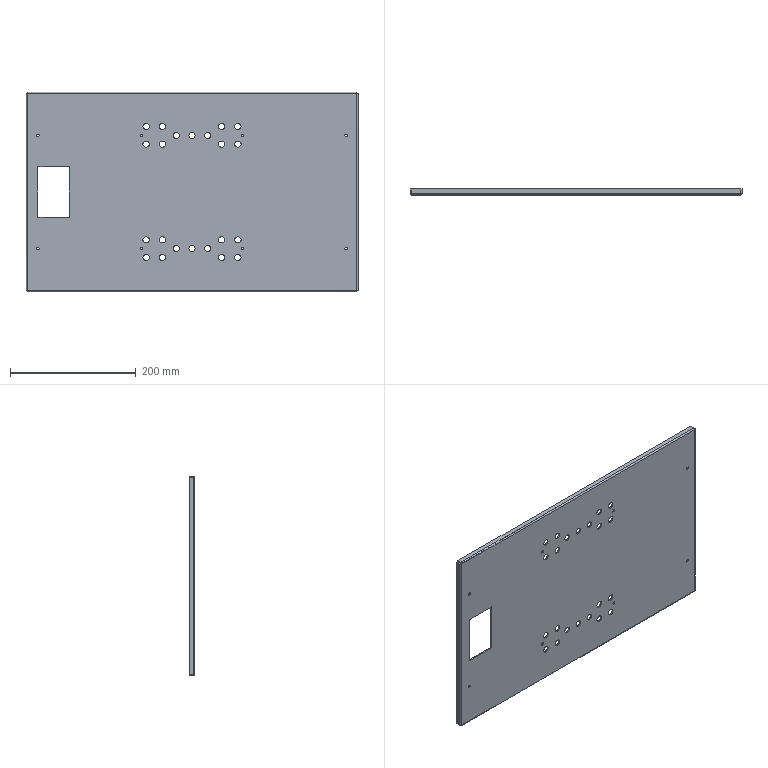Part | SolidWorks | features BaseBody 1 | 1 solid | 102 faces | box 528 x 9 x 318 mm | volume 345577 mm3 | cylinder 52 | plane 26 | cone 16 | spline 8 | commonest cylinder face diameters 10 x44 0.4 x4 4.4 x4